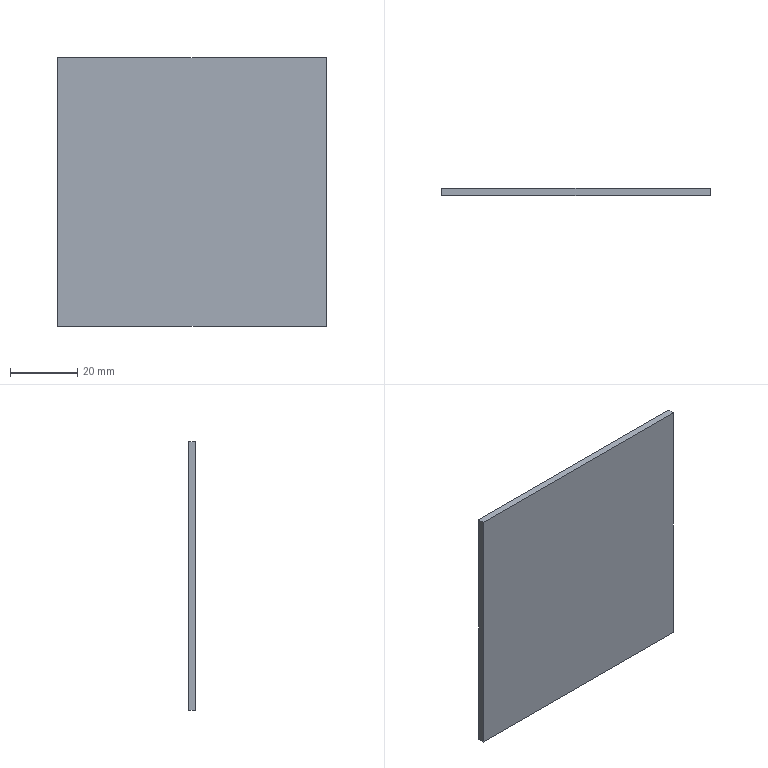Part | SolidWorks | features Extrusion 1 | 1 solid | 6 faces | box 80 x 2 x 80 mm | volume 12800 mm3 | plane 6
STEP:
#1=CARTESIAN_POINT('',(40.,0.,40.));
#2=VERTEX_POINT('',#1);
#3=CARTESIAN_POINT('',(40.,0.,-40.));
#4=VERTEX_POINT('',#3);
#5=CARTESIAN_POINT('',(40.,0.,-40.));
#6=DIRECTION('',(0.,0.,-1.));
#7=VECTOR('',#6,1000.);
#8=LINE('',#5,#7);
#9=EDGE_CURVE('',#2,#4,#8,.T.);
#10=ORIENTED_EDGE('',*,*,#9,.T.);
#11=CARTESIAN_POINT('',(40.,2.,-40.));
#12=VERTEX_POINT('',#11);
#13=CARTESIAN_POINT('',(40.,2.,-40.));
#14=DIRECTION('',(0.,-1.,0.));
#15=VECTOR('',#14,1000.);
#16=LINE('',#13,#15);
#17=EDGE_CURVE('',#12,#4,#16,.T.);
#18=ORIENTED_EDGE('',*,*,#17,.F.);
#19=CARTESIAN_POINT('',(40.,2.,40.));
#20=VERTEX_POINT('',#19);
#21=CARTESIAN_POINT('',(40.,2.,-40.));
#22=DIRECTION('',(0.,0.,-1.));
#23=VECTOR('',#22,1000.);
#24=LINE('',#21,#23);
#25=EDGE_CURVE('',#20,#12,#24,.T.);
#26=ORIENTED_EDGE('',*,*,#25,.F.);
#27=CARTESIAN_POINT('',(40.,2.,40.));
#28=DIRECTION('',(0.,-1.,0.));
#29=VECTOR('',#28,1000.);
#30=LINE('',#27,#29);
#31=EDGE_CURVE('',#20,#2,#30,.T.);
#32=ORIENTED_EDGE('',*,*,#31,.T.);
#33=EDGE_LOOP('',(#10,#18,#26,#32));
#34=FACE_OUTER_BOUND('',#33,.T.);
#35=CARTESIAN_POINT('',(40.,2.,-40.));
#36=DIRECTION('',(-1.,0.,0.));
#37=DIRECTION('',(0.,0.,1.));
#38=AXIS2_PLACEMENT_3D('',#35,#36,#37);
#39=PLANE('',#38);
#40=ADVANCED_FACE('',(#34),#39,.F.);
#41=CARTESIAN_POINT('',(-40.,0.,-40.));
#42=VERTEX_POINT('',#41);
#43=CARTESIAN_POINT('',(-40.,0.,-40.));
#44=DIRECTION('',(-1.,0.,0.));
#45=VECTOR('',#44,1000.);
#46=LINE('',#43,#45);
#47=EDGE_CURVE('',#4,#42,#46,.T.);
#48=ORIENTED_EDGE('',*,*,#47,.T.);
#49=CARTESIAN_POINT('',(-40.,2.,-40.));
#50=VERTEX_POINT('',#49);
#51=CARTESIAN_POINT('',(-40.,2.,-40.));
#52=DIRECTION('',(0.,-1.,0.));
#53=VECTOR('',#52,1000.);
#54=LINE('',#51,#53);
#55=EDGE_CURVE('',#50,#42,#54,.T.);
#56=ORIENTED_EDGE('',*,*,#55,.F.);
#57=CARTESIAN_POINT('',(-40.,2.,-40.));
#58=DIRECTION('',(-1.,0.,0.));
#59=VECTOR('',#58,1000.);
#60=LINE('',#57,#59);
#61=EDGE_CURVE('',#12,#50,#60,.T.);
#62=ORIENTED_EDGE('',*,*,#61,.F.);
#63=ORIENTED_EDGE('',*,*,#17,.T.);
#64=EDGE_LOOP('',(#48,#56,#62,#63));
#65=FACE_OUTER_BOUND('',#64,.T.);
#66=CARTESIAN_POINT('',(-40.,2.,-40.));
#67=DIRECTION('',(0.,0.,1.));
#68=DIRECTION('',(1.,0.,0.));
#69=AXIS2_PLACEMENT_3D('',#66,#67,#68);
#70=PLANE('',#69);
#71=ADVANCED_FACE('',(#65),#70,.F.);
#72=CARTESIAN_POINT('',(-40.,0.,40.));
#73=VERTEX_POINT('',#72);
#74=CARTESIAN_POINT('',(-40.,0.,-40.));
#75=DIRECTION('',(0.,0.,1.));
#76=VECTOR('',#75,1000.);
#77=LINE('',#74,#76);
#78=EDGE_CURVE('',#42,#73,#77,.T.);
#79=ORIENTED_EDGE('',*,*,#78,.T.);
#80=CARTESIAN_POINT('',(-40.,2.,40.));
#81=VERTEX_POINT('',#80);
#82=CARTESIAN_POINT('',(-40.,2.,40.));
#83=DIRECTION('',(0.,-1.,0.));
#84=VECTOR('',#83,1000.);
#85=LINE('',#82,#84);
#86=EDGE_CURVE('',#81,#73,#85,.T.);
#87=ORIENTED_EDGE('',*,*,#86,.F.);
#88=CARTESIAN_POINT('',(-40.,2.,-40.));
#89=DIRECTION('',(0.,0.,1.));
#90=VECTOR('',#89,1000.);
#91=LINE('',#88,#90);
#92=EDGE_CURVE('',#50,#81,#91,.T.);
#93=ORIENTED_EDGE('',*,*,#92,.F.);
#94=ORIENTED_EDGE('',*,*,#55,.T.);
#95=EDGE_LOOP('',(#79,#87,#93,#94));
#96=FACE_OUTER_BOUND('',#95,.T.);
#97=CARTESIAN_POINT('',(-40.,2.,-40.));
#98=DIRECTION('',(1.,0.,0.));
#99=DIRECTION('',(0.,0.,-1.));
#100=AXIS2_PLACEMENT_3D('',#97,#98,#99);
#101=PLANE('',#100);
#102=ADVANCED_FACE('',(#96),#101,.F.);
#103=CARTESIAN_POINT('',(-40.,0.,40.));
#104=DIRECTION('',(1.,0.,0.));
#105=VECTOR('',#104,1000.);
#106=LINE('',#103,#105);
#107=EDGE_CURVE('',#73,#2,#106,.T.);
#108=ORIENTED_EDGE('',*,*,#107,.T.);
#109=ORIENTED_EDGE('',*,*,#31,.F.);
#110=CARTESIAN_POINT('',(-40.,2.,40.));
#111=DIRECTION('',(1.,0.,0.));
#112=VECTOR('',#111,1000.);
#113=LINE('',#110,#112);
#114=EDGE_CURVE('',#81,#20,#113,.T.);
#115=ORIENTED_EDGE('',*,*,#114,.F.);
#116=ORIENTED_EDGE('',*,*,#86,.T.);
#117=EDGE_LOOP('',(#108,#109,#115,#116));
#118=FACE_OUTER_BOUND('',#117,.T.);
#119=CARTESIAN_POINT('',(-40.,2.,40.));
#120=DIRECTION('',(0.,0.,-1.));
#121=DIRECTION('',(-1.,0.,0.));
#122=AXIS2_PLACEMENT_3D('',#119,#120,#121);
#123=PLANE('',#122);
#124=ADVANCED_FACE('',(#118),#123,.F.);
#125=ORIENTED_EDGE('',*,*,#25,.T.);
#126=ORIENTED_EDGE('',*,*,#61,.T.);
#127=ORIENTED_EDGE('',*,*,#92,.T.);
#128=ORIENTED_EDGE('',*,*,#114,.T.);
#129=EDGE_LOOP('',(#125,#126,#127,#128));
#130=FACE_OUTER_BOUND('',#129,.T.);
#131=CARTESIAN_POINT('',(0.,2.,0.));
#132=DIRECTION('',(0.,1.,0.));
#133=DIRECTION('',(0.,0.,1.));
#134=AXIS2_PLACEMENT_3D('',#131,#132,#133);
#135=PLANE('',#134);
#136=ADVANCED_FACE('',(#130),#135,.T.);
#137=ORIENTED_EDGE('',*,*,#9,.F.);
#138=ORIENTED_EDGE('',*,*,#107,.F.);
#139=ORIENTED_EDGE('',*,*,#78,.F.);
#140=ORIENTED_EDGE('',*,*,#47,.F.);
#141=EDGE_LOOP('',(#137,#138,#139,#140));
#142=FACE_OUTER_BOUND('',#141,.T.);
#143=CARTESIAN_POINT('',(0.,0.,0.));
#144=DIRECTION('',(0.,1.,0.));
#145=DIRECTION('',(0.,0.,1.));
#146=AXIS2_PLACEMENT_3D('',#143,#144,#145);
#147=PLANE('',#146);
#148=ADVANCED_FACE('',(#142),#147,.F.);
#149=CLOSED_SHELL('',(#40,#71,#102,#124,#136,#148));
#150=MANIFOLD_SOLID_BREP('',#149);
#151=CARTESIAN_POINT('',(0.,0.,0.));
#152=DIRECTION('',(0.,0.,1.));
#153=DIRECTION('',(1.,0.,0.));
#154=AXIS2_PLACEMENT_3D('',#151,#152,#153);
#155=(LENGTH_UNIT()NAMED_UNIT(*)SI_UNIT(.MILLI.,.METRE.));
#156=UNCERTAINTY_MEASURE_WITH_UNIT(LENGTH_MEASURE(0.00001),#155,'','');
#157=(NAMED_UNIT(*)PLANE_ANGLE_UNIT()SI_UNIT($,.RADIAN.));
#158=(NAMED_UNIT(*)SI_UNIT($,.STERADIAN.)SOLID_ANGLE_UNIT());
#159=(GEOMETRIC_REPRESENTATION_CONTEXT(3)GLOBAL_UNCERTAINTY_ASSIGNED_CONTEXT((#156))GLOBAL_UNIT_ASSIGNED_CONTEXT((#155,#157,#158))REPRESENTATION_CONTEXT('',''));
#160=ADVANCED_BREP_SHAPE_REPRESENTATION('',(#150,#154),#159);